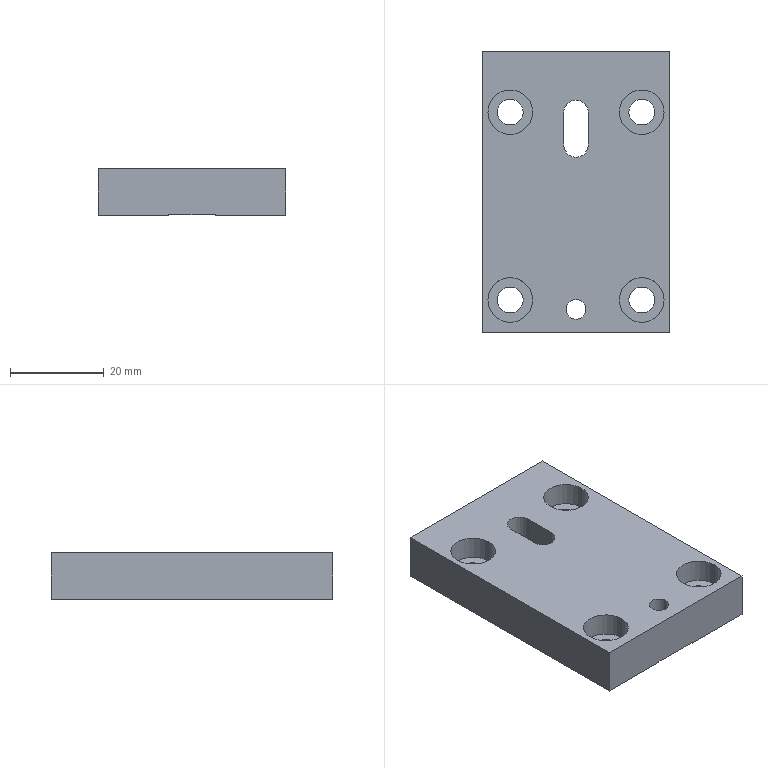Part | STEP file | BU-C06-1 | 1 solid | 36 faces | box 40 x 60 x 10 mm | volume 21287 mm3 | cylinder 20 | plane 16 | commonest cylinder face diameters 5.5 x8 9.5 x8 4.2 x2 5.2 x2